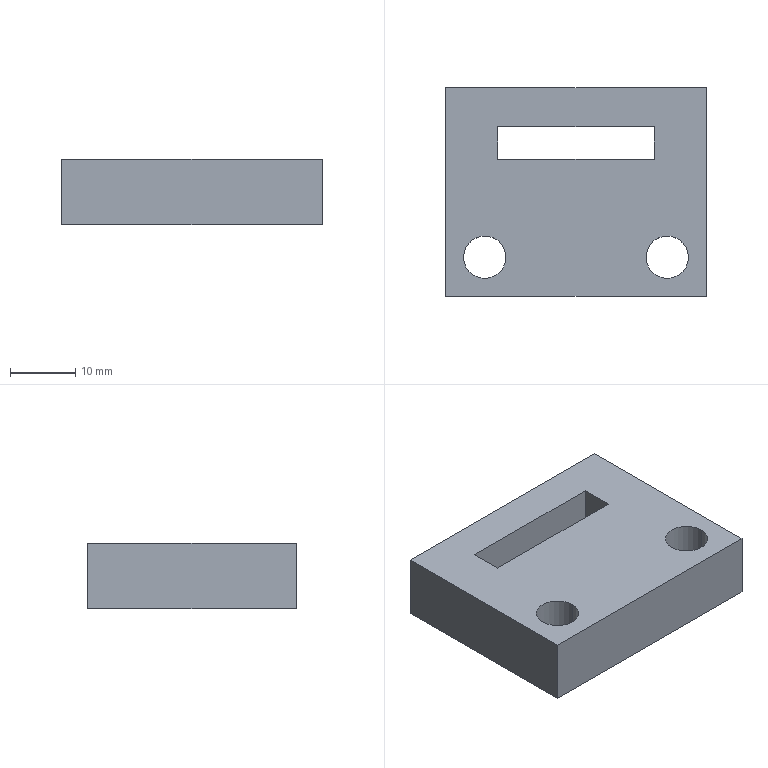Part | 1 solid | 14 faces | box 40 x 32 x 10 mm | volume 10244 mm3 | plane 10 | cylinder 4 | commonest cylinder face diameters 6.5 x4
STEP:
#1=CARTESIAN_POINT('',(10.75,0.,10.));
#2=VERTEX_POINT('',#1);
#3=CARTESIAN_POINT('',(17.25,0.,10.));
#4=VERTEX_POINT('',#3);
#5=CARTESIAN_POINT('',(14.,0.,10.));
#6=DIRECTION('',(0.,0.,1.));
#7=DIRECTION('',(1.,0.,0.));
#8=AXIS2_PLACEMENT_3D('',#5,#6,#7);
#9=CIRCLE('',#8,3.25);
#10=EDGE_CURVE('',#2,#4,#9,.T.);
#11=ORIENTED_EDGE('',*,*,#10,.T.);
#12=CARTESIAN_POINT('',(17.25,0.,0.));
#13=VERTEX_POINT('',#12);
#14=CARTESIAN_POINT('',(17.25,0.,10.));
#15=DIRECTION('',(0.,0.,-1.));
#16=VECTOR('',#15,1000.);
#17=LINE('',#14,#16);
#18=EDGE_CURVE('',#4,#13,#17,.T.);
#19=ORIENTED_EDGE('',*,*,#18,.T.);
#20=CARTESIAN_POINT('',(10.75,0.,0.));
#21=VERTEX_POINT('',#20);
#22=CARTESIAN_POINT('',(14.,0.,0.));
#23=DIRECTION('',(0.,0.,1.));
#24=DIRECTION('',(1.,0.,0.));
#25=AXIS2_PLACEMENT_3D('',#22,#23,#24);
#26=CIRCLE('',#25,3.25);
#27=EDGE_CURVE('',#21,#13,#26,.T.);
#28=ORIENTED_EDGE('',*,*,#27,.F.);
#29=CARTESIAN_POINT('',(10.75,0.,10.));
#30=DIRECTION('',(0.,0.,-1.));
#31=VECTOR('',#30,1000.);
#32=LINE('',#29,#31);
#33=EDGE_CURVE('',#2,#21,#32,.T.);
#34=ORIENTED_EDGE('',*,*,#33,.F.);
#35=EDGE_LOOP('',(#11,#19,#28,#34));
#36=FACE_OUTER_BOUND('',#35,.T.);
#37=CARTESIAN_POINT('',(14.,0.,10.));
#38=DIRECTION('',(0.,0.,-1.));
#39=DIRECTION('',(-1.,0.,0.));
#40=AXIS2_PLACEMENT_3D('',#37,#38,#39);
#41=CYLINDRICAL_SURFACE('',#40,3.25);
#42=ADVANCED_FACE('',(#36),#41,.F.);
#43=CARTESIAN_POINT('',(-17.25,0.,10.));
#44=VERTEX_POINT('',#43);
#45=CARTESIAN_POINT('',(-10.75,0.,10.));
#46=VERTEX_POINT('',#45);
#47=CARTESIAN_POINT('',(-14.,0.,10.));
#48=DIRECTION('',(0.,0.,1.));
#49=DIRECTION('',(1.,0.,0.));
#50=AXIS2_PLACEMENT_3D('',#47,#48,#49);
#51=CIRCLE('',#50,3.25);
#52=EDGE_CURVE('',#44,#46,#51,.T.);
#53=ORIENTED_EDGE('',*,*,#52,.T.);
#54=CARTESIAN_POINT('',(-10.75,0.,0.));
#55=VERTEX_POINT('',#54);
#56=CARTESIAN_POINT('',(-10.75,0.,10.));
#57=DIRECTION('',(0.,0.,-1.));
#58=VECTOR('',#57,1000.);
#59=LINE('',#56,#58);
#60=EDGE_CURVE('',#46,#55,#59,.T.);
#61=ORIENTED_EDGE('',*,*,#60,.T.);
#62=CARTESIAN_POINT('',(-17.25,0.,0.));
#63=VERTEX_POINT('',#62);
#64=CARTESIAN_POINT('',(-14.,0.,0.));
#65=DIRECTION('',(0.,0.,1.));
#66=DIRECTION('',(1.,0.,0.));
#67=AXIS2_PLACEMENT_3D('',#64,#65,#66);
#68=CIRCLE('',#67,3.25);
#69=EDGE_CURVE('',#63,#55,#68,.T.);
#70=ORIENTED_EDGE('',*,*,#69,.F.);
#71=CARTESIAN_POINT('',(-17.25,0.,10.));
#72=DIRECTION('',(0.,0.,-1.));
#73=VECTOR('',#72,1000.);
#74=LINE('',#71,#73);
#75=EDGE_CURVE('',#44,#63,#74,.T.);
#76=ORIENTED_EDGE('',*,*,#75,.F.);
#77=EDGE_LOOP('',(#53,#61,#70,#76));
#78=FACE_OUTER_BOUND('',#77,.T.);
#79=CARTESIAN_POINT('',(-14.,0.,10.));
#80=DIRECTION('',(0.,0.,-1.));
#81=DIRECTION('',(-1.,0.,0.));
#82=AXIS2_PLACEMENT_3D('',#79,#80,#81);
#83=CYLINDRICAL_SURFACE('',#82,3.25);
#84=ADVANCED_FACE('',(#78),#83,.F.);
#85=CARTESIAN_POINT('',(20.,-6.,10.));
#86=VERTEX_POINT('',#85);
#87=CARTESIAN_POINT('',(20.,26.,10.));
#88=VERTEX_POINT('',#87);
#89=CARTESIAN_POINT('',(20.,-6.,10.));
#90=DIRECTION('',(0.,1.,0.));
#91=VECTOR('',#90,1000.);
#92=LINE('',#89,#91);
#93=EDGE_CURVE('',#86,#88,#92,.T.);
#94=ORIENTED_EDGE('',*,*,#93,.T.);
#95=CARTESIAN_POINT('',(-20.,26.,10.));
#96=VERTEX_POINT('',#95);
#97=CARTESIAN_POINT('',(-20.,26.,10.));
#98=DIRECTION('',(-1.,0.,0.));
#99=VECTOR('',#98,1000.);
#100=LINE('',#97,#99);
#101=EDGE_CURVE('',#88,#96,#100,.T.);
#102=ORIENTED_EDGE('',*,*,#101,.T.);
#103=CARTESIAN_POINT('',(-20.,-6.,10.));
#104=VERTEX_POINT('',#103);
#105=CARTESIAN_POINT('',(-20.,-6.,10.));
#106=DIRECTION('',(0.,-1.,0.));
#107=VECTOR('',#106,1000.);
#108=LINE('',#105,#107);
#109=EDGE_CURVE('',#96,#104,#108,.T.);
#110=ORIENTED_EDGE('',*,*,#109,.T.);
#111=CARTESIAN_POINT('',(-20.,-6.,10.));
#112=DIRECTION('',(1.,0.,0.));
#113=VECTOR('',#112,1000.);
#114=LINE('',#111,#113);
#115=EDGE_CURVE('',#104,#86,#114,.T.);
#116=ORIENTED_EDGE('',*,*,#115,.T.);
#117=EDGE_LOOP('',(#94,#102,#110,#116));
#118=FACE_OUTER_BOUND('',#117,.T.);
#119=ORIENTED_EDGE('',*,*,#52,.F.);
#120=CARTESIAN_POINT('',(-14.,0.,10.));
#121=DIRECTION('',(0.,0.,1.));
#122=DIRECTION('',(1.,0.,0.));
#123=AXIS2_PLACEMENT_3D('',#120,#121,#122);
#124=CIRCLE('',#123,3.25);
#125=EDGE_CURVE('',#46,#44,#124,.T.);
#126=ORIENTED_EDGE('',*,*,#125,.F.);
#127=EDGE_LOOP('',(#119,#126));
#128=FACE_BOUND('',#127,.T.);
#129=ORIENTED_EDGE('',*,*,#10,.F.);
#130=CARTESIAN_POINT('',(14.,0.,10.));
#131=DIRECTION('',(0.,0.,1.));
#132=DIRECTION('',(1.,0.,0.));
#133=AXIS2_PLACEMENT_3D('',#130,#131,#132);
#134=CIRCLE('',#133,3.25);
#135=EDGE_CURVE('',#4,#2,#134,.T.);
#136=ORIENTED_EDGE('',*,*,#135,.F.);
#137=EDGE_LOOP('',(#129,#136));
#138=FACE_BOUND('',#137,.T.);
#139=CARTESIAN_POINT('',(-12.,15.,10.));
#140=VERTEX_POINT('',#139);
#141=CARTESIAN_POINT('',(12.,15.,10.));
#142=VERTEX_POINT('',#141);
#143=CARTESIAN_POINT('',(-12.,15.,10.));
#144=DIRECTION('',(1.,0.,0.));
#145=VECTOR('',#144,1000.);
#146=LINE('',#143,#145);
#147=EDGE_CURVE('',#140,#142,#146,.T.);
#148=ORIENTED_EDGE('',*,*,#147,.F.);
#149=CARTESIAN_POINT('',(-12.,20.,10.));
#150=VERTEX_POINT('',#149);
#151=CARTESIAN_POINT('',(-12.,20.,10.));
#152=DIRECTION('',(0.,-1.,0.));
#153=VECTOR('',#152,1000.);
#154=LINE('',#151,#153);
#155=EDGE_CURVE('',#150,#140,#154,.T.);
#156=ORIENTED_EDGE('',*,*,#155,.F.);
#157=CARTESIAN_POINT('',(12.,20.,10.));
#158=VERTEX_POINT('',#157);
#159=CARTESIAN_POINT('',(-12.,20.,10.));
#160=DIRECTION('',(-1.,0.,0.));
#161=VECTOR('',#160,1000.);
#162=LINE('',#159,#161);
#163=EDGE_CURVE('',#158,#150,#162,.T.);
#164=ORIENTED_EDGE('',*,*,#163,.F.);
#165=CARTESIAN_POINT('',(12.,20.,10.));
#166=DIRECTION('',(0.,1.,0.));
#167=VECTOR('',#166,1000.);
#168=LINE('',#165,#167);
#169=EDGE_CURVE('',#142,#158,#168,.T.);
#170=ORIENTED_EDGE('',*,*,#169,.F.);
#171=EDGE_LOOP('',(#148,#156,#164,#170));
#172=FACE_BOUND('',#171,.T.);
#173=CARTESIAN_POINT('',(0.,0.,10.));
#174=DIRECTION('',(0.,0.,-1.));
#175=DIRECTION('',(-1.,0.,0.));
#176=AXIS2_PLACEMENT_3D('',#173,#174,#175);
#177=PLANE('',#176);
#178=ADVANCED_FACE('',(#118,#128,#138,#172),#177,.F.);
#179=ORIENTED_EDGE('',*,*,#69,.T.);
#180=CARTESIAN_POINT('',(-14.,0.,0.));
#181=DIRECTION('',(0.,0.,1.));
#182=DIRECTION('',(1.,0.,0.));
#183=AXIS2_PLACEMENT_3D('',#180,#181,#182);
#184=CIRCLE('',#183,3.25);
#185=EDGE_CURVE('',#55,#63,#184,.T.);
#186=ORIENTED_EDGE('',*,*,#185,.T.);
#187=EDGE_LOOP('',(#179,#186));
#188=FACE_BOUND('',#187,.T.);
#189=CARTESIAN_POINT('',(20.,-6.,0.));
#190=VERTEX_POINT('',#189);
#191=CARTESIAN_POINT('',(20.,26.,0.));
#192=VERTEX_POINT('',#191);
#193=CARTESIAN_POINT('',(20.,-6.,0.));
#194=DIRECTION('',(0.,1.,0.));
#195=VECTOR('',#194,1000.);
#196=LINE('',#193,#195);
#197=EDGE_CURVE('',#190,#192,#196,.T.);
#198=ORIENTED_EDGE('',*,*,#197,.F.);
#199=CARTESIAN_POINT('',(-20.,-6.,0.));
#200=VERTEX_POINT('',#199);
#201=CARTESIAN_POINT('',(-20.,-6.,0.));
#202=DIRECTION('',(1.,0.,0.));
#203=VECTOR('',#202,1000.);
#204=LINE('',#201,#203);
#205=EDGE_CURVE('',#200,#190,#204,.T.);
#206=ORIENTED_EDGE('',*,*,#205,.F.);
#207=CARTESIAN_POINT('',(-20.,26.,0.));
#208=VERTEX_POINT('',#207);
#209=CARTESIAN_POINT('',(-20.,-6.,0.));
#210=DIRECTION('',(0.,-1.,0.));
#211=VECTOR('',#210,1000.);
#212=LINE('',#209,#211);
#213=EDGE_CURVE('',#208,#200,#212,.T.);
#214=ORIENTED_EDGE('',*,*,#213,.F.);
#215=CARTESIAN_POINT('',(-20.,26.,0.));
#216=DIRECTION('',(-1.,0.,0.));
#217=VECTOR('',#216,1000.);
#218=LINE('',#215,#217);
#219=EDGE_CURVE('',#192,#208,#218,.T.);
#220=ORIENTED_EDGE('',*,*,#219,.F.);
#221=EDGE_LOOP('',(#198,#206,#214,#220));
#222=FACE_OUTER_BOUND('',#221,.T.);
#223=ORIENTED_EDGE('',*,*,#27,.T.);
#224=CARTESIAN_POINT('',(14.,0.,0.));
#225=DIRECTION('',(0.,0.,1.));
#226=DIRECTION('',(1.,0.,0.));
#227=AXIS2_PLACEMENT_3D('',#224,#225,#226);
#228=CIRCLE('',#227,3.25);
#229=EDGE_CURVE('',#13,#21,#228,.T.);
#230=ORIENTED_EDGE('',*,*,#229,.T.);
#231=EDGE_LOOP('',(#223,#230));
#232=FACE_BOUND('',#231,.T.);
#233=CARTESIAN_POINT('',(-12.,9.226,0.));
#234=VERTEX_POINT('',#233);
#235=CARTESIAN_POINT('',(12.,9.226,0.));
#236=VERTEX_POINT('',#235);
#237=CARTESIAN_POINT('',(12.,9.226,0.));
#238=DIRECTION('',(1.,0.,0.));
#239=VECTOR('',#238,1000.);
#240=LINE('',#237,#239);
#241=EDGE_CURVE('',#234,#236,#240,.T.);
#242=ORIENTED_EDGE('',*,*,#241,.T.);
#243=CARTESIAN_POINT('',(12.,20.,0.));
#244=VERTEX_POINT('',#243);
#245=CARTESIAN_POINT('',(12.,20.,0.));
#246=DIRECTION('',(0.,1.,0.));
#247=VECTOR('',#246,1000.);
#248=LINE('',#245,#247);
#249=EDGE_CURVE('',#236,#244,#248,.T.);
#250=ORIENTED_EDGE('',*,*,#249,.T.);
#251=CARTESIAN_POINT('',(-12.,20.,0.));
#252=VERTEX_POINT('',#251);
#253=CARTESIAN_POINT('',(-12.,20.,0.));
#254=DIRECTION('',(-1.,0.,0.));
#255=VECTOR('',#254,1000.);
#256=LINE('',#253,#255);
#257=EDGE_CURVE('',#244,#252,#256,.T.);
#258=ORIENTED_EDGE('',*,*,#257,.T.);
#259=CARTESIAN_POINT('',(-12.,20.,0.));
#260=DIRECTION('',(0.,-1.,0.));
#261=VECTOR('',#260,1000.);
#262=LINE('',#259,#261);
#263=EDGE_CURVE('',#252,#234,#262,.T.);
#264=ORIENTED_EDGE('',*,*,#263,.T.);
#265=EDGE_LOOP('',(#242,#250,#258,#264));
#266=FACE_BOUND('',#265,.T.);
#267=CARTESIAN_POINT('',(0.,0.,0.));
#268=DIRECTION('',(0.,0.,-1.));
#269=DIRECTION('',(-1.,0.,0.));
#270=AXIS2_PLACEMENT_3D('',#267,#268,#269);
#271=PLANE('',#270);
#272=ADVANCED_FACE('',(#188,#222,#232,#266),#271,.T.);
#273=ORIENTED_EDGE('',*,*,#197,.T.);
#274=CARTESIAN_POINT('',(20.,26.,-44.721));
#275=DIRECTION('',(0.,0.,1.));
#276=VECTOR('',#275,1000.);
#277=LINE('',#274,#276);
#278=EDGE_CURVE('',#192,#88,#277,.T.);
#279=ORIENTED_EDGE('',*,*,#278,.T.);
#280=ORIENTED_EDGE('',*,*,#93,.F.);
#281=CARTESIAN_POINT('',(20.,-6.,10.));
#282=DIRECTION('',(0.,0.,-1.));
#283=VECTOR('',#282,1000.);
#284=LINE('',#281,#283);
#285=EDGE_CURVE('',#86,#190,#284,.T.);
#286=ORIENTED_EDGE('',*,*,#285,.T.);
#287=EDGE_LOOP('',(#273,#279,#280,#286));
#288=FACE_OUTER_BOUND('',#287,.T.);
#289=CARTESIAN_POINT('',(20.,-6.,10.));
#290=DIRECTION('',(-1.,0.,0.));
#291=DIRECTION('',(0.,0.,1.));
#292=AXIS2_PLACEMENT_3D('',#289,#290,#291);
#293=PLANE('',#292);
#294=ADVANCED_FACE('',(#288),#293,.F.);
#295=ORIENTED_EDGE('',*,*,#213,.T.);
#296=CARTESIAN_POINT('',(-20.,-6.,10.));
#297=DIRECTION('',(0.,0.,-1.));
#298=VECTOR('',#297,1000.);
#299=LINE('',#296,#298);
#300=EDGE_CURVE('',#104,#200,#299,.T.);
#301=ORIENTED_EDGE('',*,*,#300,.F.);
#302=ORIENTED_EDGE('',*,*,#109,.F.);
#303=CARTESIAN_POINT('',(-20.,26.,-44.721));
#304=DIRECTION('',(0.,0.,1.));
#305=VECTOR('',#304,1000.);
#306=LINE('',#303,#305);
#307=EDGE_CURVE('',#208,#96,#306,.T.);
#308=ORIENTED_EDGE('',*,*,#307,.F.);
#309=EDGE_LOOP('',(#295,#301,#302,#308));
#310=FACE_OUTER_BOUND('',#309,.T.);
#311=CARTESIAN_POINT('',(-20.,-6.,10.));
#312=DIRECTION('',(1.,0.,0.));
#313=DIRECTION('',(0.,0.,-1.));
#314=AXIS2_PLACEMENT_3D('',#311,#312,#313);
#315=PLANE('',#314);
#316=ADVANCED_FACE('',(#310),#315,.F.);
#317=ORIENTED_EDGE('',*,*,#205,.T.);
#318=ORIENTED_EDGE('',*,*,#285,.F.);
#319=ORIENTED_EDGE('',*,*,#115,.F.);
#320=ORIENTED_EDGE('',*,*,#300,.T.);
#321=EDGE_LOOP('',(#317,#318,#319,#320));
#322=FACE_OUTER_BOUND('',#321,.T.);
#323=CARTESIAN_POINT('',(-20.,-6.,10.));
#324=DIRECTION('',(0.,1.,0.));
#325=DIRECTION('',(0.,0.,1.));
#326=AXIS2_PLACEMENT_3D('',#323,#324,#325);
#327=PLANE('',#326);
#328=ADVANCED_FACE('',(#322),#327,.F.);
#329=ORIENTED_EDGE('',*,*,#60,.F.);
#330=ORIENTED_EDGE('',*,*,#125,.T.);
#331=ORIENTED_EDGE('',*,*,#75,.T.);
#332=ORIENTED_EDGE('',*,*,#185,.F.);
#333=EDGE_LOOP('',(#329,#330,#331,#332));
#334=FACE_OUTER_BOUND('',#333,.T.);
#335=CARTESIAN_POINT('',(-14.,0.,10.));
#336=DIRECTION('',(0.,0.,-1.));
#337=DIRECTION('',(-1.,0.,0.));
#338=AXIS2_PLACEMENT_3D('',#335,#336,#337);
#339=CYLINDRICAL_SURFACE('',#338,3.25);
#340=ADVANCED_FACE('',(#334),#339,.F.);
#341=ORIENTED_EDGE('',*,*,#18,.F.);
#342=ORIENTED_EDGE('',*,*,#135,.T.);
#343=ORIENTED_EDGE('',*,*,#33,.T.);
#344=ORIENTED_EDGE('',*,*,#229,.F.);
#345=EDGE_LOOP('',(#341,#342,#343,#344));
#346=FACE_OUTER_BOUND('',#345,.T.);
#347=CARTESIAN_POINT('',(14.,0.,10.));
#348=DIRECTION('',(0.,0.,-1.));
#349=DIRECTION('',(-1.,0.,0.));
#350=AXIS2_PLACEMENT_3D('',#347,#348,#349);
#351=CYLINDRICAL_SURFACE('',#350,3.25);
#352=ADVANCED_FACE('',(#346),#351,.F.);
#353=ORIENTED_EDGE('',*,*,#278,.F.);
#354=ORIENTED_EDGE('',*,*,#219,.T.);
#355=ORIENTED_EDGE('',*,*,#307,.T.);
#356=ORIENTED_EDGE('',*,*,#101,.F.);
#357=EDGE_LOOP('',(#353,#354,#355,#356));
#358=FACE_OUTER_BOUND('',#357,.T.);
#359=CARTESIAN_POINT('',(-20.,26.,-44.721));
#360=DIRECTION('',(0.,1.,0.));
#361=DIRECTION('',(0.,0.,1.));
#362=AXIS2_PLACEMENT_3D('',#359,#360,#361);
#363=PLANE('',#362);
#364=ADVANCED_FACE('',(#358),#363,.T.);
#365=ORIENTED_EDGE('',*,*,#263,.F.);
#366=CARTESIAN_POINT('',(-12.,20.,-44.721));
#367=DIRECTION('',(0.,0.,1.));
#368=VECTOR('',#367,1000.);
#369=LINE('',#366,#368);
#370=EDGE_CURVE('',#252,#150,#369,.T.);
#371=ORIENTED_EDGE('',*,*,#370,.T.);
#372=ORIENTED_EDGE('',*,*,#155,.T.);
#373=CARTESIAN_POINT('',(-12.,-7.445,-28.876));
#374=DIRECTION('',(0.,-0.5,-0.866));
#375=VECTOR('',#374,1000.);
#376=LINE('',#373,#375);
#377=EDGE_CURVE('',#140,#234,#376,.T.);
#378=ORIENTED_EDGE('',*,*,#377,.T.);
#379=EDGE_LOOP('',(#365,#371,#372,#378));
#380=FACE_OUTER_BOUND('',#379,.T.);
#381=CARTESIAN_POINT('',(-12.,20.,-44.721));
#382=DIRECTION('',(-1.,0.,0.));
#383=DIRECTION('',(0.,-1.,0.));
#384=AXIS2_PLACEMENT_3D('',#381,#382,#383);
#385=PLANE('',#384);
#386=ADVANCED_FACE('',(#380),#385,.F.);
#387=ORIENTED_EDGE('',*,*,#257,.F.);
#388=CARTESIAN_POINT('',(12.,20.,-44.721));
#389=DIRECTION('',(0.,0.,1.));
#390=VECTOR('',#389,1000.);
#391=LINE('',#388,#390);
#392=EDGE_CURVE('',#244,#158,#391,.T.);
#393=ORIENTED_EDGE('',*,*,#392,.T.);
#394=ORIENTED_EDGE('',*,*,#163,.T.);
#395=ORIENTED_EDGE('',*,*,#370,.F.);
#396=EDGE_LOOP('',(#387,#393,#394,#395));
#397=FACE_OUTER_BOUND('',#396,.T.);
#398=CARTESIAN_POINT('',(-12.,20.,-44.721));
#399=DIRECTION('',(0.,1.,0.));
#400=DIRECTION('',(0.,0.,1.));
#401=AXIS2_PLACEMENT_3D('',#398,#399,#400);
#402=PLANE('',#401);
#403=ADVANCED_FACE('',(#397),#402,.F.);
#404=ORIENTED_EDGE('',*,*,#249,.F.);
#405=CARTESIAN_POINT('',(12.,-7.445,-28.876));
#406=DIRECTION('',(0.,0.5,0.866));
#407=VECTOR('',#406,1000.);
#408=LINE('',#405,#407);
#409=EDGE_CURVE('',#236,#142,#408,.T.);
#410=ORIENTED_EDGE('',*,*,#409,.T.);
#411=ORIENTED_EDGE('',*,*,#169,.T.);
#412=ORIENTED_EDGE('',*,*,#392,.F.);
#413=EDGE_LOOP('',(#404,#410,#411,#412));
#414=FACE_OUTER_BOUND('',#413,.T.);
#415=CARTESIAN_POINT('',(12.,20.,-44.721));
#416=DIRECTION('',(1.,0.,0.));
#417=DIRECTION('',(0.,1.,0.));
#418=AXIS2_PLACEMENT_3D('',#415,#416,#417);
#419=PLANE('',#418);
#420=ADVANCED_FACE('',(#414),#419,.F.);
#421=ORIENTED_EDGE('',*,*,#377,.F.);
#422=ORIENTED_EDGE('',*,*,#147,.T.);
#423=ORIENTED_EDGE('',*,*,#409,.F.);
#424=ORIENTED_EDGE('',*,*,#241,.F.);
#425=EDGE_LOOP('',(#421,#422,#423,#424));
#426=FACE_OUTER_BOUND('',#425,.T.);
#427=CARTESIAN_POINT('',(0.,9.226,0.));
#428=DIRECTION('',(0.,0.866,-0.5));
#429=DIRECTION('',(-1.,0.,0.));
#430=AXIS2_PLACEMENT_3D('',#427,#428,#429);
#431=PLANE('',#430);
#432=ADVANCED_FACE('',(#426),#431,.T.);
#433=CLOSED_SHELL('',(#42,#84,#178,#272,#294,#316,#328,#340,#352,#364,#386,#403,#420,#432));
#434=MANIFOLD_SOLID_BREP('',#433);
#435=CARTESIAN_POINT('',(0.,0.,0.));
#436=DIRECTION('',(0.,0.,1.));
#437=DIRECTION('',(1.,0.,0.));
#438=AXIS2_PLACEMENT_3D('',#435,#436,#437);
#439=(LENGTH_UNIT()NAMED_UNIT(*)SI_UNIT(.MILLI.,.METRE.));
#440=UNCERTAINTY_MEASURE_WITH_UNIT(LENGTH_MEASURE(0.00001),#439,'','');
#441=(NAMED_UNIT(*)PLANE_ANGLE_UNIT()SI_UNIT($,.RADIAN.));
#442=(NAMED_UNIT(*)SI_UNIT($,.STERADIAN.)SOLID_ANGLE_UNIT());
#443=(GEOMETRIC_REPRESENTATION_CONTEXT(3)GLOBAL_UNCERTAINTY_ASSIGNED_CONTEXT((#440))GLOBAL_UNIT_ASSIGNED_CONTEXT((#439,#441,#442))REPRESENTATION_CONTEXT('',''));
#444=ADVANCED_BREP_SHAPE_REPRESENTATION('',(#434,#438),#443);